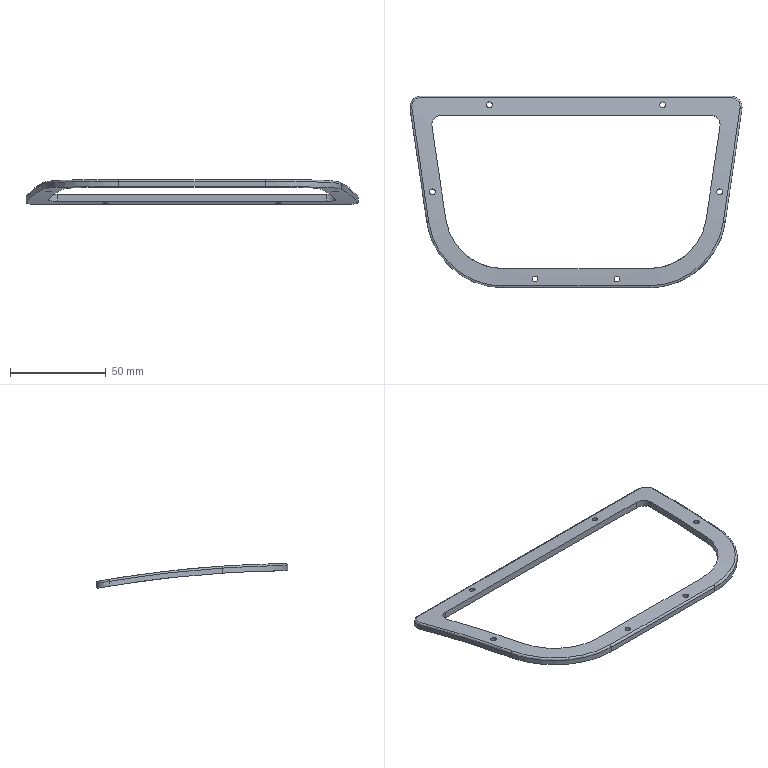Part | SolidWorks | features SplitBody 1 | 1 solid | 40 faces | box 173.097 x 99.841 x 12.86 mm | volume 16352 mm3 | cylinder 24 | plane 8 | spline 8 | commonest cylinder face diameters 3 x12 10 x3 12 x3 2 x2 60 x2 80 x2